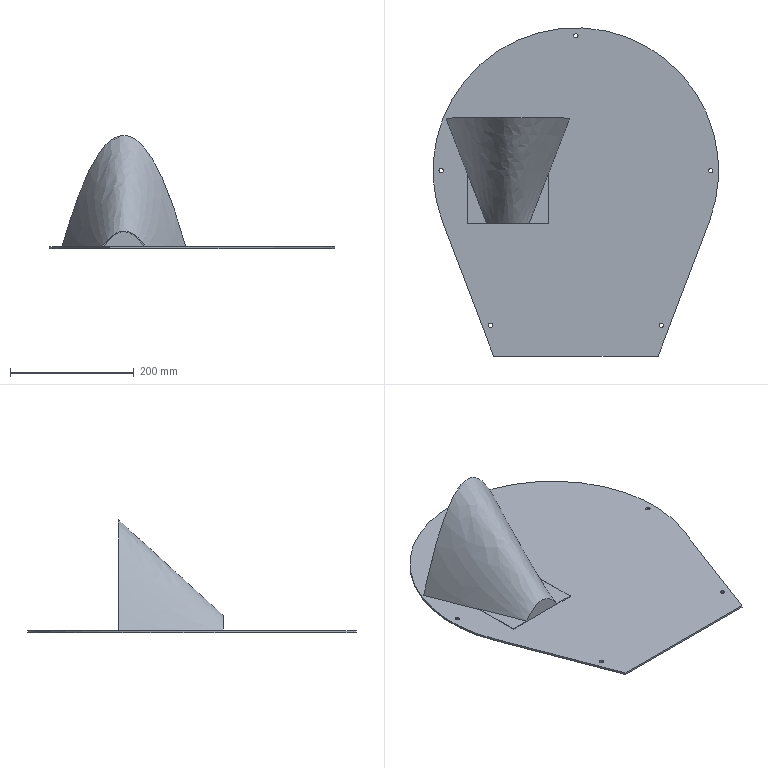Part | SolidWorks | features AEMSimFeature 1 | 1 solid | 29 faces | box 462 x 531 x 183 mm | volume 626105 mm3 | plane 15 | cylinder 12 | spline 2 | commonest cylinder face diameters 7 x10 462 x2